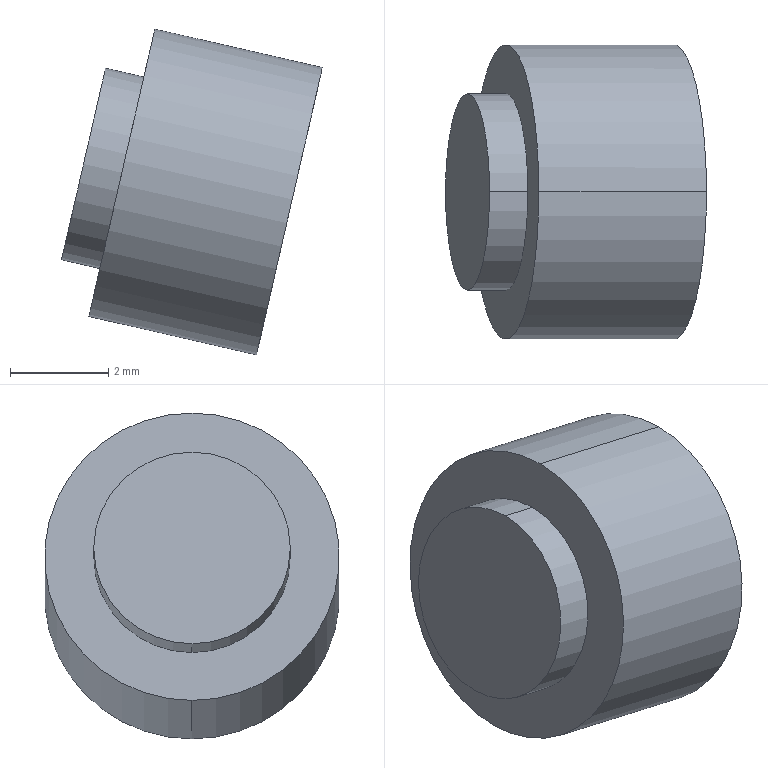Part | SolidWorks | features BaseBody 1 | 1 solid | 10 faces | box 5.31 x 6 x 6.631 mm | volume 70.058 mm3 | cylinder 6 | plane 4 | commonest cylinder face diameters 4 x4 6 x2
STEP:
#1=CARTESIAN_POINT('',(1990.041,-186.778,916.434));
#2=VERTEX_POINT('',#1);
#3=CARTESIAN_POINT('',(1989.145,-186.778,912.536));
#4=VERTEX_POINT('',#3);
#5=CARTESIAN_POINT('',(1989.593,-186.778,914.485));
#6=DIRECTION('',(0.9746,0.,-0.2239));
#7=DIRECTION('',(0.2239,0.,0.9746));
#8=AXIS2_PLACEMENT_3D('',#5,#6,#7);
#9=CIRCLE('',#8,2.);
#10=EDGE_CURVE('',#2,#4,#9,.T.);
#11=ORIENTED_EDGE('',*,*,#10,.T.);
#12=CARTESIAN_POINT('',(1986.124,-186.778,913.23));
#13=VERTEX_POINT('',#12);
#14=CARTESIAN_POINT('',(1991.777,-186.778,911.931));
#15=DIRECTION('',(-0.9746,0.,0.2239));
#16=VECTOR('',#15,1000.);
#17=LINE('',#14,#16);
#18=EDGE_CURVE('',#4,#13,#17,.T.);
#19=ORIENTED_EDGE('',*,*,#18,.T.);
#20=CARTESIAN_POINT('',(1987.02,-186.778,917.128));
#21=VERTEX_POINT('',#20);
#22=CARTESIAN_POINT('',(1986.572,-186.778,915.179));
#23=DIRECTION('',(0.9746,0.,-0.2239));
#24=DIRECTION('',(0.2239,0.,0.9746));
#25=AXIS2_PLACEMENT_3D('',#22,#23,#24);
#26=CIRCLE('',#25,2.);
#27=EDGE_CURVE('',#21,#13,#26,.T.);
#28=ORIENTED_EDGE('',*,*,#27,.F.);
#29=CARTESIAN_POINT('',(1992.672,-186.778,915.83));
#30=DIRECTION('',(-0.9746,0.,0.2239));
#31=VECTOR('',#30,1000.);
#32=LINE('',#29,#31);
#33=EDGE_CURVE('',#2,#21,#32,.T.);
#34=ORIENTED_EDGE('',*,*,#33,.F.);
#35=EDGE_LOOP('',(#11,#19,#28,#34));
#36=FACE_OUTER_BOUND('',#35,.T.);
#37=CARTESIAN_POINT('',(1992.225,-186.778,913.88));
#38=DIRECTION('',(-0.9746,0.,0.2239));
#39=DIRECTION('',(0.2239,0.,0.9746));
#40=AXIS2_PLACEMENT_3D('',#37,#38,#39);
#41=CYLINDRICAL_SURFACE('',#40,2.);
#42=ADVANCED_FACE('',(#36),#41,.F.);
#43=CARTESIAN_POINT('',(1990.265,-186.778,917.409));
#44=VERTEX_POINT('',#43);
#45=CARTESIAN_POINT('',(1988.922,-186.778,911.561));
#46=VERTEX_POINT('',#45);
#47=CARTESIAN_POINT('',(1989.593,-186.778,914.485));
#48=DIRECTION('',(-0.9746,0.,0.2239));
#49=DIRECTION('',(-0.2239,0.,-0.9746));
#50=AXIS2_PLACEMENT_3D('',#47,#48,#49);
#51=CIRCLE('',#50,3.);
#52=EDGE_CURVE('',#44,#46,#51,.T.);
#53=ORIENTED_EDGE('',*,*,#52,.T.);
#54=CARTESIAN_POINT('',(1985.51,-186.778,912.344));
#55=VERTEX_POINT('',#54);
#56=CARTESIAN_POINT('',(1988.922,-186.778,911.561));
#57=DIRECTION('',(-0.9746,0.,0.2239));
#58=VECTOR('',#57,1000.);
#59=LINE('',#56,#58);
#60=EDGE_CURVE('',#46,#55,#59,.T.);
#61=ORIENTED_EDGE('',*,*,#60,.T.);
#62=CARTESIAN_POINT('',(1986.854,-186.778,918.192));
#63=VERTEX_POINT('',#62);
#64=CARTESIAN_POINT('',(1986.182,-186.778,915.268));
#65=DIRECTION('',(-0.9746,0.,0.2239));
#66=DIRECTION('',(0.2239,0.,0.9746));
#67=AXIS2_PLACEMENT_3D('',#64,#65,#66);
#68=CIRCLE('',#67,3.);
#69=EDGE_CURVE('',#63,#55,#68,.T.);
#70=ORIENTED_EDGE('',*,*,#69,.F.);
#71=CARTESIAN_POINT('',(1990.265,-186.778,917.409));
#72=DIRECTION('',(-0.9746,0.,0.2239));
#73=VECTOR('',#72,1000.);
#74=LINE('',#71,#73);
#75=EDGE_CURVE('',#44,#63,#74,.T.);
#76=ORIENTED_EDGE('',*,*,#75,.F.);
#77=EDGE_LOOP('',(#53,#61,#70,#76));
#78=FACE_OUTER_BOUND('',#77,.T.);
#79=CARTESIAN_POINT('',(1989.593,-186.778,914.485));
#80=DIRECTION('',(-0.9746,0.,0.2239));
#81=DIRECTION('',(0.2239,0.,0.9746));
#82=AXIS2_PLACEMENT_3D('',#79,#80,#81);
#83=CYLINDRICAL_SURFACE('',#82,3.);
#84=ADVANCED_FACE('',(#78),#83,.T.);
#85=CARTESIAN_POINT('',(1986.63,-186.778,917.218));
#86=VERTEX_POINT('',#85);
#87=CARTESIAN_POINT('',(1985.734,-186.778,913.319));
#88=VERTEX_POINT('',#87);
#89=CARTESIAN_POINT('',(1986.182,-186.778,915.268));
#90=DIRECTION('',(-0.9746,0.,0.2239));
#91=DIRECTION('',(-0.2239,0.,-0.9746));
#92=AXIS2_PLACEMENT_3D('',#89,#90,#91);
#93=CIRCLE('',#92,2.);
#94=EDGE_CURVE('',#86,#88,#93,.T.);
#95=ORIENTED_EDGE('',*,*,#94,.T.);
#96=CARTESIAN_POINT('',(1984.955,-186.778,913.498));
#97=VERTEX_POINT('',#96);
#98=CARTESIAN_POINT('',(1985.734,-186.778,913.319));
#99=DIRECTION('',(-0.9746,0.,0.2239));
#100=VECTOR('',#99,1000.);
#101=LINE('',#98,#100);
#102=EDGE_CURVE('',#88,#97,#101,.T.);
#103=ORIENTED_EDGE('',*,*,#102,.T.);
#104=CARTESIAN_POINT('',(1985.85,-186.778,917.397));
#105=VERTEX_POINT('',#104);
#106=CARTESIAN_POINT('',(1985.402,-186.778,915.447));
#107=DIRECTION('',(-0.9746,0.,0.2239));
#108=DIRECTION('',(0.2239,0.,0.9746));
#109=AXIS2_PLACEMENT_3D('',#106,#107,#108);
#110=CIRCLE('',#109,2.);
#111=EDGE_CURVE('',#105,#97,#110,.T.);
#112=ORIENTED_EDGE('',*,*,#111,.F.);
#113=CARTESIAN_POINT('',(1986.63,-186.778,917.218));
#114=DIRECTION('',(-0.9746,0.,0.2239));
#115=VECTOR('',#114,1000.);
#116=LINE('',#113,#115);
#117=EDGE_CURVE('',#86,#105,#116,.T.);
#118=ORIENTED_EDGE('',*,*,#117,.F.);
#119=EDGE_LOOP('',(#95,#103,#112,#118));
#120=FACE_OUTER_BOUND('',#119,.T.);
#121=CARTESIAN_POINT('',(1986.182,-186.778,915.268));
#122=DIRECTION('',(-0.9746,0.,0.2239));
#123=DIRECTION('',(0.2239,0.,0.9746));
#124=AXIS2_PLACEMENT_3D('',#121,#122,#123);
#125=CYLINDRICAL_SURFACE('',#124,2.);
#126=ADVANCED_FACE('',(#120),#125,.T.);
#127=ORIENTED_EDGE('',*,*,#52,.F.);
#128=CARTESIAN_POINT('',(1989.593,-186.778,914.485));
#129=DIRECTION('',(-0.9746,0.,0.2239));
#130=DIRECTION('',(-0.2239,0.,-0.9746));
#131=AXIS2_PLACEMENT_3D('',#128,#129,#130);
#132=CIRCLE('',#131,3.);
#133=EDGE_CURVE('',#46,#44,#132,.T.);
#134=ORIENTED_EDGE('',*,*,#133,.F.);
#135=EDGE_LOOP('',(#127,#134));
#136=FACE_OUTER_BOUND('',#135,.T.);
#137=ORIENTED_EDGE('',*,*,#10,.F.);
#138=CARTESIAN_POINT('',(1989.593,-186.778,914.485));
#139=DIRECTION('',(0.9746,0.,-0.2239));
#140=DIRECTION('',(0.2239,0.,0.9746));
#141=AXIS2_PLACEMENT_3D('',#138,#139,#140);
#142=CIRCLE('',#141,2.);
#143=EDGE_CURVE('',#4,#2,#142,.T.);
#144=ORIENTED_EDGE('',*,*,#143,.F.);
#145=EDGE_LOOP('',(#137,#144));
#146=FACE_BOUND('',#145,.T.);
#147=CARTESIAN_POINT('',(1989.593,-186.778,914.485));
#148=DIRECTION('',(-0.9746,0.,0.2239));
#149=DIRECTION('',(0.2239,0.,0.9746));
#150=AXIS2_PLACEMENT_3D('',#147,#148,#149);
#151=PLANE('',#150);
#152=ADVANCED_FACE('',(#136,#146),#151,.F.);
#153=ORIENTED_EDGE('',*,*,#102,.F.);
#154=CARTESIAN_POINT('',(1986.182,-186.778,915.268));
#155=DIRECTION('',(-0.9746,0.,0.2239));
#156=DIRECTION('',(-0.2239,0.,-0.9746));
#157=AXIS2_PLACEMENT_3D('',#154,#155,#156);
#158=CIRCLE('',#157,2.);
#159=EDGE_CURVE('',#88,#86,#158,.T.);
#160=ORIENTED_EDGE('',*,*,#159,.T.);
#161=ORIENTED_EDGE('',*,*,#117,.T.);
#162=CARTESIAN_POINT('',(1985.402,-186.778,915.447));
#163=DIRECTION('',(-0.9746,0.,0.2239));
#164=DIRECTION('',(0.2239,0.,0.9746));
#165=AXIS2_PLACEMENT_3D('',#162,#163,#164);
#166=CIRCLE('',#165,2.);
#167=EDGE_CURVE('',#97,#105,#166,.T.);
#168=ORIENTED_EDGE('',*,*,#167,.F.);
#169=EDGE_LOOP('',(#153,#160,#161,#168));
#170=FACE_OUTER_BOUND('',#169,.T.);
#171=CARTESIAN_POINT('',(1986.182,-186.778,915.268));
#172=DIRECTION('',(-0.9746,0.,0.2239));
#173=DIRECTION('',(0.2239,0.,0.9746));
#174=AXIS2_PLACEMENT_3D('',#171,#172,#173);
#175=CYLINDRICAL_SURFACE('',#174,2.);
#176=ADVANCED_FACE('',(#170),#175,.T.);
#177=ORIENTED_EDGE('',*,*,#111,.T.);
#178=ORIENTED_EDGE('',*,*,#167,.T.);
#179=EDGE_LOOP('',(#177,#178));
#180=FACE_OUTER_BOUND('',#179,.T.);
#181=CARTESIAN_POINT('',(1985.402,-186.778,915.447));
#182=DIRECTION('',(-0.9746,0.,0.2239));
#183=DIRECTION('',(0.2239,0.,0.9746));
#184=AXIS2_PLACEMENT_3D('',#181,#182,#183);
#185=PLANE('',#184);
#186=ADVANCED_FACE('',(#180),#185,.T.);
#187=ORIENTED_EDGE('',*,*,#69,.T.);
#188=CARTESIAN_POINT('',(1986.182,-186.778,915.268));
#189=DIRECTION('',(-0.9746,0.,0.2239));
#190=DIRECTION('',(0.2239,0.,0.9746));
#191=AXIS2_PLACEMENT_3D('',#188,#189,#190);
#192=CIRCLE('',#191,3.);
#193=EDGE_CURVE('',#55,#63,#192,.T.);
#194=ORIENTED_EDGE('',*,*,#193,.T.);
#195=EDGE_LOOP('',(#187,#194));
#196=FACE_OUTER_BOUND('',#195,.T.);
#197=ORIENTED_EDGE('',*,*,#94,.F.);
#198=ORIENTED_EDGE('',*,*,#159,.F.);
#199=EDGE_LOOP('',(#197,#198));
#200=FACE_BOUND('',#199,.T.);
#201=CARTESIAN_POINT('',(1986.182,-186.778,915.268));
#202=DIRECTION('',(-0.9746,0.,0.2239));
#203=DIRECTION('',(0.2239,0.,0.9746));
#204=AXIS2_PLACEMENT_3D('',#201,#202,#203);
#205=PLANE('',#204);
#206=ADVANCED_FACE('',(#196,#200),#205,.T.);
#207=ORIENTED_EDGE('',*,*,#60,.F.);
#208=ORIENTED_EDGE('',*,*,#133,.T.);
#209=ORIENTED_EDGE('',*,*,#75,.T.);
#210=ORIENTED_EDGE('',*,*,#193,.F.);
#211=EDGE_LOOP('',(#207,#208,#209,#210));
#212=FACE_OUTER_BOUND('',#211,.T.);
#213=CARTESIAN_POINT('',(1989.593,-186.778,914.485));
#214=DIRECTION('',(-0.9746,0.,0.2239));
#215=DIRECTION('',(0.2239,0.,0.9746));
#216=AXIS2_PLACEMENT_3D('',#213,#214,#215);
#217=CYLINDRICAL_SURFACE('',#216,3.);
#218=ADVANCED_FACE('',(#212),#217,.T.);
#219=ORIENTED_EDGE('',*,*,#18,.F.);
#220=ORIENTED_EDGE('',*,*,#143,.T.);
#221=ORIENTED_EDGE('',*,*,#33,.T.);
#222=CARTESIAN_POINT('',(1986.572,-186.778,915.179));
#223=DIRECTION('',(0.9746,0.,-0.2239));
#224=DIRECTION('',(0.2239,0.,0.9746));
#225=AXIS2_PLACEMENT_3D('',#222,#223,#224);
#226=CIRCLE('',#225,2.);
#227=EDGE_CURVE('',#13,#21,#226,.T.);
#228=ORIENTED_EDGE('',*,*,#227,.F.);
#229=EDGE_LOOP('',(#219,#220,#221,#228));
#230=FACE_OUTER_BOUND('',#229,.T.);
#231=CARTESIAN_POINT('',(1992.225,-186.778,913.88));
#232=DIRECTION('',(-0.9746,0.,0.2239));
#233=DIRECTION('',(0.2239,0.,0.9746));
#234=AXIS2_PLACEMENT_3D('',#231,#232,#233);
#235=CYLINDRICAL_SURFACE('',#234,2.);
#236=ADVANCED_FACE('',(#230),#235,.F.);
#237=ORIENTED_EDGE('',*,*,#27,.T.);
#238=ORIENTED_EDGE('',*,*,#227,.T.);
#239=EDGE_LOOP('',(#237,#238));
#240=FACE_OUTER_BOUND('',#239,.T.);
#241=CARTESIAN_POINT('',(1986.572,-186.778,915.179));
#242=DIRECTION('',(0.9746,0.,-0.2239));
#243=DIRECTION('',(-0.2239,0.,-0.9746));
#244=AXIS2_PLACEMENT_3D('',#241,#242,#243);
#245=PLANE('',#244);
#246=ADVANCED_FACE('',(#240),#245,.T.);
#247=CLOSED_SHELL('',(#42,#84,#126,#152,#176,#186,#206,#218,#236,#246));
#248=MANIFOLD_SOLID_BREP('',#247);
#249=CARTESIAN_POINT('',(0.,0.,0.));
#250=DIRECTION('',(0.,0.,1.));
#251=DIRECTION('',(1.,0.,0.));
#252=AXIS2_PLACEMENT_3D('',#249,#250,#251);
#253=(LENGTH_UNIT()NAMED_UNIT(*)SI_UNIT(.MILLI.,.METRE.));
#254=UNCERTAINTY_MEASURE_WITH_UNIT(LENGTH_MEASURE(0.00001),#253,'','');
#255=(NAMED_UNIT(*)PLANE_ANGLE_UNIT()SI_UNIT($,.RADIAN.));
#256=(NAMED_UNIT(*)SI_UNIT($,.STERADIAN.)SOLID_ANGLE_UNIT());
#257=(GEOMETRIC_REPRESENTATION_CONTEXT(3)GLOBAL_UNCERTAINTY_ASSIGNED_CONTEXT((#254))GLOBAL_UNIT_ASSIGNED_CONTEXT((#253,#255,#256))REPRESENTATION_CONTEXT('',''));
#258=ADVANCED_BREP_SHAPE_REPRESENTATION('',(#248,#252),#257);